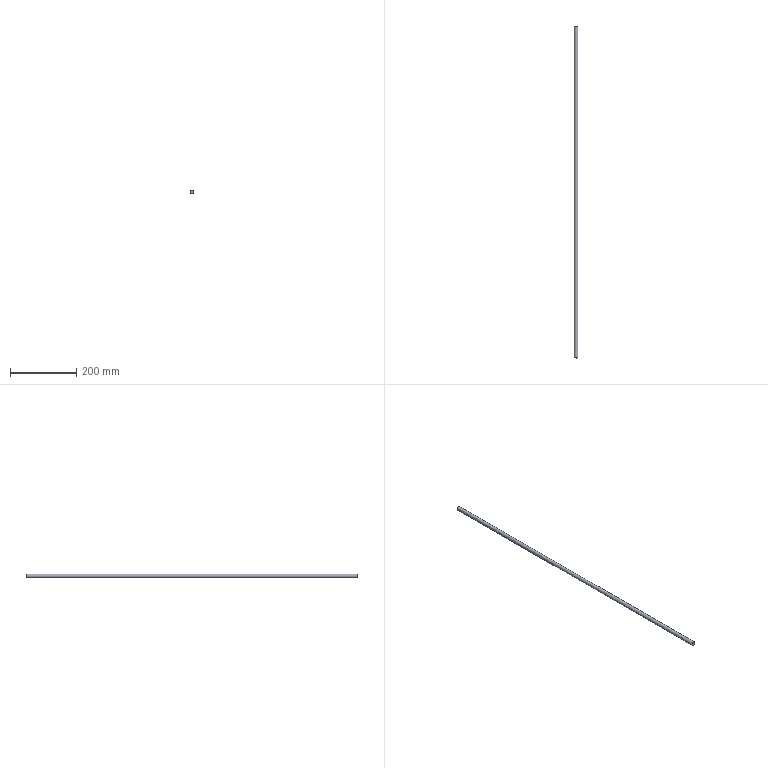Part | STEP file | solid 177 | 1 solid | 3 faces | box 12 x 1000 x 12 mm | volume 113097 mm3 | plane 2 | cylinder 1 | commonest cylinder face diameters 12 x1